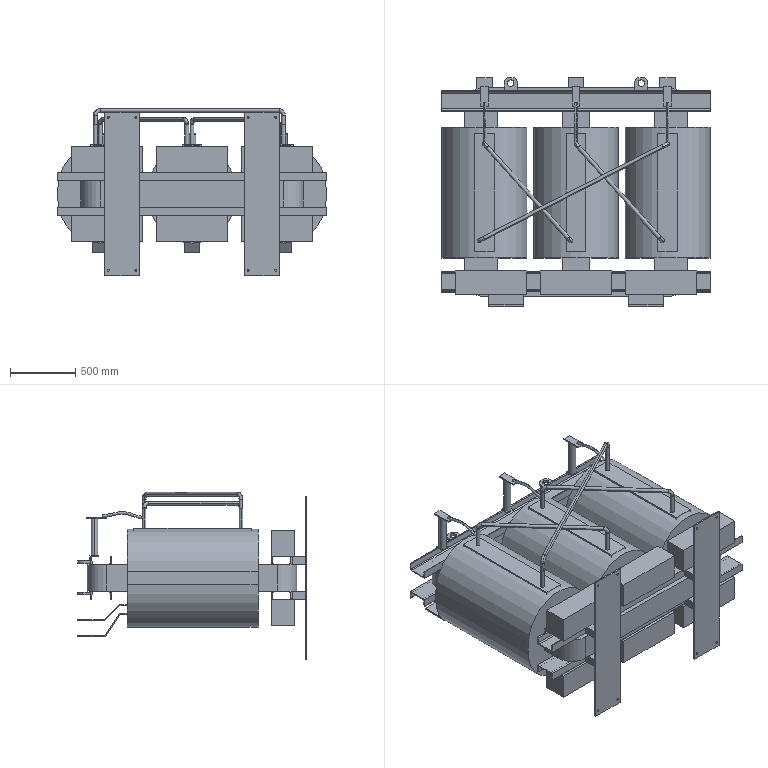Part | STEP file | 400-TX-103_default<by machining> | 51 solids | 536 faces | box 2050 x 1750 x 1280 mm | volume 1654351010 mm3 | plane 381 | cylinder 91 | spline 56 | torus 8 | commonest cylinder face diameters 14 x16 29.368 x12 30 x12 650 x9 10 x8 20 x8